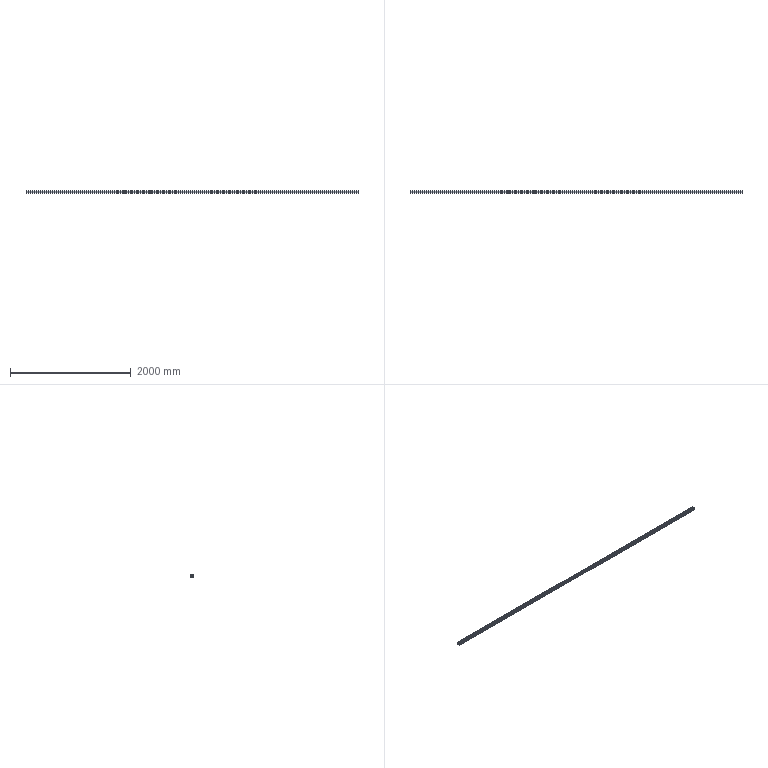Part | STEP file | 1_1 | 1 solid | 87 faces | box 5510 x 45 x 45 mm | volume 4505764 mm3 | plane 78 | cylinder 9 | commonest cylinder face diameters 2 x4 6 x4 10 x1